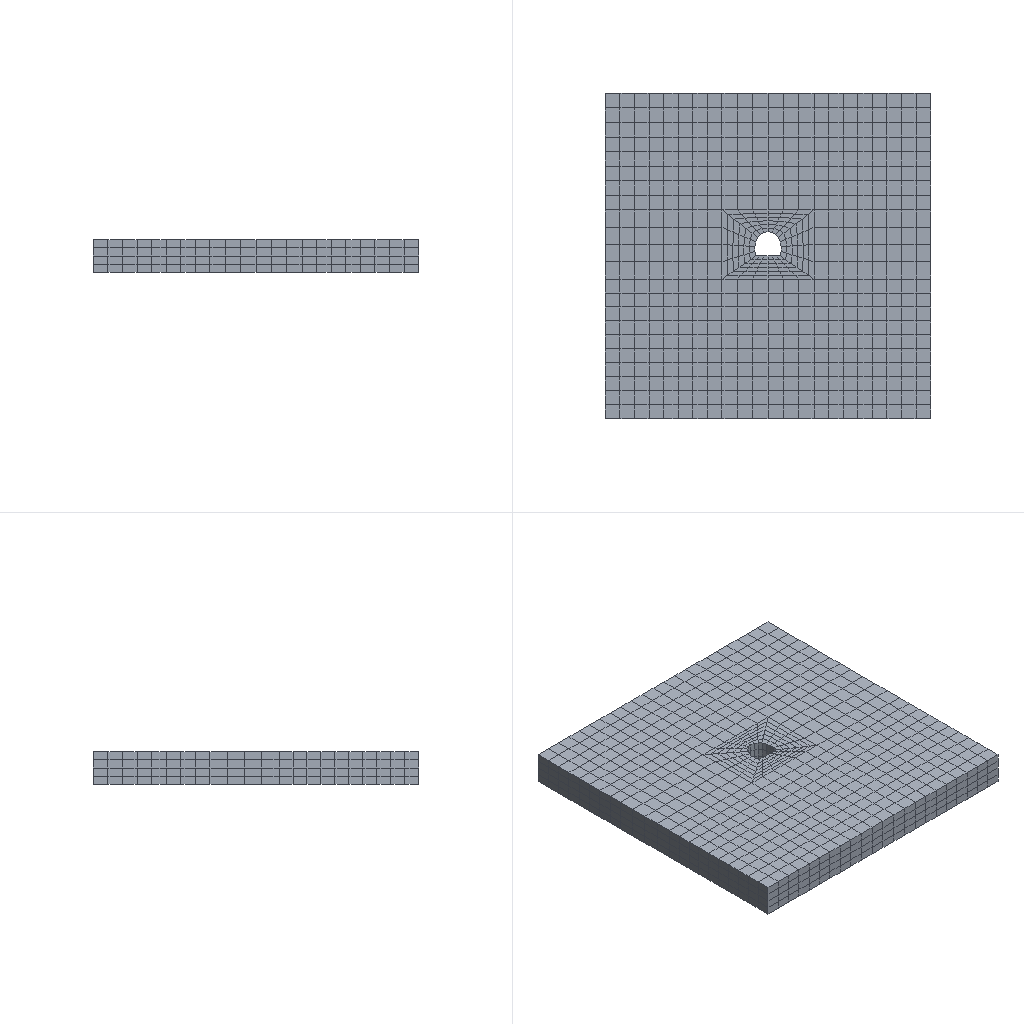Simulation study | abaqus
Set-up summary:
category,name,step,type,value,unit,region
solver,abaqus
solver,version,,,Abaqus/Standard 2020
units,not stated in the deck,,not stated
analysis,deck,,geostatic,geostatic; soils
load_step,Step-1,Step-1,geostatic,nlgeom=False
load_step,Step-2,Step-2,soils,nlgeom=False
contact,interactions,,,general=0 pairs=0 ties=0
load_step,requested,,,2
mesh,nodes,,,3170
mesh,elements,,,2320
element_type,C3D8PT,,solid,2320
load,load commands in deck,,count,1
bc,support commands in deck,,count,4
material,MATERIAL-1,,in results
check,setup vs results,,match,"per instance, exact: element labels, types and connectivity; labels of the nodes the elements use; coordinates of those nodes at SINGLE_PRECISION in 1 of 1 instance(s)"
Abaqus input file, long lists of numbers shortened:
*Heading
** Job name: Job-1 Model name: Job-try7
** Generated by: Abaqus/CAE 2020
*Preprint, echo=NO, model=NO, history=NO, contact=NO
**
** PARTS
**
*Part, name=PART-2
*Node
      1,   14.16,  -7.097,           0.
      2,   14.16,         -50.,           0.
** (3168 more lines like these left out)
*Element, type=C3D8PT
   1,  102,  597, 1893,  567,    1,   41,  477,   68
   2,  597,  598, 1894, 1893,   41,   42,  478,  477
** (2318 more lines like these left out)
*Nset, nset=_PICKEDSET2, internal, generate
    1,  3170,     1
*Elset, elset=_PICKEDSET2, internal, generate
    1,  2320,     1
** Section: Section-1-_PICKEDSET2
*Solid Section, elset=_PICKEDSET2, material=MATERIAL-1
,
*End Part
**
**
** ASSEMBLY
**
*Assembly, name=Assembly
**
*Instance, name=PART-2-1, part=PART-2
*End Instance
**
*Nset, nset=Set-12, instance=PART-2-1, generate
    1,  3170,     1
*Nset, nset=Set-13, instance=PART-2-1
   10,   11,   13,   14,   25,   26,   27,   28,  114,  115,  116,  130,  131,  132,  151,  152
  153,  154,  155,  156,  157,  158,  159,  160,  260,  261,  262,  268,  269,  270,  271,  272
** (5 more lines like these left out)
*Nset, nset=Set-14, instance=PART-2-1
   10,   11,   13,   14,   25,   26,   27,   28,  114,  115,  116,  130,  131,  132,  151,  152
  153,  154,  155,  156,  157,  158,  159,  160,  260,  261,  262,  268,  269,  270,  271,  272
** (5 more lines like these left out)
*Nset, nset=Set-15, instance=PART-2-1, generate
    1,  3170,     1
*Nset, nset=Set-16, instance=PART-2-1
   29,   30,   31,   32,   35,   36,   37,   38,  299,  300,  301,  302,  303,  304,  305,  306
  307,  308,  309,  310,  356,  357,  358,  359,  360,  361,  362,  363,  364,  365,  366,  367
** (6 more lines like these left out)
*Nset, nset=Set-17, instance=PART-2-1
    2,    3,    5,    6,   37,   38,   39,   40,   50,   51,   52,   53,   54,   78,   79,   80
   81,   82,  103,  104,  105,  106,  107,  108,  396,  397,  398,  408,  409,  410,  411,  412
** (6 more lines like these left out)
*Nset, nset=Set-18, instance=PART-2-1
    1,    2,    3,    4,    9,   10,   13,   16,   17,   18,   21,   24,   25,   27,   29,   30
   33,   35,   37,   39,   41,   42,   43,   44,   45,   46,   47,   48,   49,   50,   51,   52
** (38 more lines like these left out)
*Nset, nset=Set-19, instance=PART-2-1, generate
    1,  3170,     1
*Nset, nset=Set-20, instance=PART-2-1
    2,    3,    5,    6,   17,   18,   19,   20,   21,   22,   23,   24,   29,   30,   31,   32
   33,   34,   35,   36,   37,   38,   39,   40,   50,   51,   52,   53,   54,   78,   79,   80
** (26 more lines like these left out)
*Nset, nset=Set-21, instance=PART-2-1
   10,   11,   13,   14,   25,   26,   27,   28,  114,  115,  116,  130,  131,  132,  151,  152
  153,  154,  155,  156,  157,  158,  159,  160,  260,  261,  262,  268,  269,  270,  271,  272
** (5 more lines like these left out)
*Nset, nset=Set-22, instance=PART-2-1
    1,    2,    3,    4,    5,    6,    7,    8,    9,   10,   11,   12,   13,   14,   15,   16
   17,   18,   19,   20,   21,   22,   23,   24,   25,   26,   27,   28,   29,   30,   31,   32
** (78 more lines like these left out)
*Nset, nset=Set-23, instance=PART-2-1
    2,    3,    5,    6,   21,   22,   23,   24,   33,   34,   35,   36,   37,   38,   39,   40
   50,   51,   52,   53,   54,   78,   79,   80,   81,   82,  103,  104,  105,  106,  107,  108
** (13 more lines like these left out)
*Nset, nset=Set-24, instance=PART-2-1
   17,   18,   19,   20,   23,   24,   29,   30,   31,   32,   35,   36,   37,   38,   39,   40
  168,  169,  170,  188,  189,  190,  201,  202,  203,  204,  205,  206,  224,  225,  226,  227
** (13 more lines like these left out)
*Nset, nset=_PICKEDSET78, internal, instance=PART-2-1
   29,   30,   31,   32,   35,   36,   37,   38,  299,  300,  301,  302,  303,  304,  305,  306
  307,  308,  309,  310,  356,  357,  358,  359,  360,  361,  362,  363,  364,  365,  366,  367
** (6 more lines like these left out)
*Elset, elset=_PICKEDSET78, internal, instance=PART-2-1
 1073, 1074, 1075, 1076, 1077, 1078, 1079, 1080, 1081, 1082, 1083, 1084, 1085, 1086, 1087, 1088
 1313, 1314, 1315, 1316, 1317, 1318, 1319, 1320, 1321, 1322, 1323, 1324, 1325, 1326, 1327, 1328
** (4 more lines like these left out)
*Nset, nset=_PICKEDSET85, internal, instance=PART-2-1
    1,    2,    3,    4,    9,   10,   13,   16,   17,   18,   21,   24,   25,   27,   29,   30
   33,   35,   37,   39,   41,   42,   43,   44,   45,   46,   47,   48,   49,   50,   51,   52
** (38 more lines like these left out)
*Elset, elset=_PICKEDSET85, internal, instance=PART-2-1
    1,    2,    3,    4,    5,    6,    7,    8,    9,   10,   11,   12,   13,   14,   15,   16
   17,   18,   19,   20,   21,   22,   23,   24,   25,   26,   27,   28,   29,   30,   31,   32
** (35 more lines like these left out)
*Nset, nset=_PICKEDSET86, internal, instance=PART-2-1
    2,    3,    5,    6,   37,   38,   39,   40,   50,   51,   52,   53,   54,   78,   79,   80
   81,   82,  103,  104,  105,  106,  107,  108,  396,  397,  398,  408,  409,  410,  411,  412
** (6 more lines like these left out)
*Elset, elset=_PICKEDSET86, internal, instance=PART-2-1
   10,   20,   30,   40,   50,   60,   70,   80,   90,  100,  110,  120,  130,  140,  150,  160
  170,  180,  190,  200,  210,  220,  230,  240, 1381, 1382, 1383, 1384, 1421, 1422, 1423, 1424
** (4 more lines like these left out)
*Elset, elset=__PICKEDSURF74_S2, internal, instance=PART-2-1, generate
 1665,  1688,     1
*Elset, elset=__PICKEDSURF74_S6, internal, instance=PART-2-1
  513,  521,  529,  537,  545,  553,  561,  569,  577,  585,  593,  601,  609,  617,  625,  633
  641,  649,  657,  665,  673,  681,  689,  697,  705,  713,  721,  729,  737,  745,  753,  761
** (2 more lines like these left out)
*Elset, elset=__PICKEDSURF75_S1, internal, instance=PART-2-1
  737,  738,  739,  740,  741,  742,  743,  744,  745,  746,  747,  748,  749,  750,  751,  752
  753,  754,  755,  756,  757,  758,  759,  760,  761,  762,  763,  764,  765,  766,  767,  768
** (3 more lines like these left out)
*Elset, elset=__PICKEDSURF75_S4, internal, instance=PART-2-1, generate
 392,  512,    8
*Elset, elset=__PICKEDSURF84_S1, internal, instance=PART-2-1
 181, 182, 183, 184, 185, 186, 187, 188, 189, 190, 191, 192, 193, 194, 195, 196
 197, 198, 199, 200, 201, 202, 203, 204, 205, 206, 207, 208, 209, 210, 211, 212
** (4 more lines like these left out)
*Elset, elset=__PICKEDSURF84_S3, internal, instance=PART-2-1
 1857, 1858, 1859, 1860, 1861, 1862, 1881, 1882, 1883, 1884, 1885, 1886, 1905, 1906, 1907, 1908
 1909, 1910, 1929, 1930, 1931, 1932, 1933, 1934, 1953, 1954, 1955, 1956, 1957, 1958, 1977, 1978
** (1 more lines like these left out)
*Elset, elset=__PICKEDSURF84_S5, internal, instance=PART-2-1
  259,  260,  261,  262,  263,  264,  283,  284,  285,  286,  287,  288,  307,  308,  309,  310
  311,  312,  331,  332,  333,  334,  335,  336,  355,  356,  357,  358,  359,  360,  379,  380
** (19 more lines like these left out)
*Elset, elset=__PICKEDSURF84_S6, internal, instance=PART-2-1, generate
 1345,  1853,     4
*Elset, elset=__PICKEDSURF74_S6_1, internal, instance=PART-2-1
  513,  521,  529,  537,  545,  553,  561,  569,  577,  585,  593,  601,  609,  617,  625,  633
  641,  649,  657,  665,  673,  681,  689,  697,  705,  713,  721,  729,  737,  745,  753,  761
** (2 more lines like these left out)
*Elset, elset=__PICKEDSURF74_S2_1, internal, instance=PART-2-1, generate
 1665,  1688,     1
*Surface, type=ELEMENT, name=_PICKEDSURF74, internal
__PICKEDSURF74_S6_1, S6
__PICKEDSURF74_S2_1, S2
*Elset, elset=__PICKEDSURF75_S1_1, internal, instance=PART-2-1
  737,  738,  739,  740,  741,  742,  743,  744,  745,  746,  747,  748,  749,  750,  751,  752
  753,  754,  755,  756,  757,  758,  759,  760,  761,  762,  763,  764,  765,  766,  767,  768
** (3 more lines like these left out)
*Elset, elset=__PICKEDSURF75_S4_1, internal, instance=PART-2-1, generate
 392,  512,    8
*Surface, type=ELEMENT, name=_PICKEDSURF75, internal
__PICKEDSURF75_S1_1, S1
__PICKEDSURF75_S4_1, S4
*Elset, elset=__PICKEDSURF84_S6_1, internal, instance=PART-2-1, generate
 1345,  1853,     4
*Elset, elset=__PICKEDSURF84_S5_1, internal, instance=PART-2-1
  259,  260,  261,  262,  263,  264,  283,  284,  285,  286,  287,  288,  307,  308,  309,  310
  311,  312,  331,  332,  333,  334,  335,  336,  355,  356,  357,  358,  359,  360,  379,  380
** (19 more lines like these left out)
*Elset, elset=__PICKEDSURF84_S1_1, internal, instance=PART-2-1
 181, 182, 183, 184, 185, 186, 187, 188, 189, 190, 191, 192, 193, 194, 195, 196
 197, 198, 199, 200, 201, 202, 203, 204, 205, 206, 207, 208, 209, 210, 211, 212
** (4 more lines like these left out)
*Elset, elset=__PICKEDSURF84_S3_1, internal, instance=PART-2-1
 1857, 1858, 1859, 1860, 1861, 1862, 1881, 1882, 1883, 1884, 1885, 1886, 1905, 1906, 1907, 1908
 1909, 1910, 1929, 1930, 1931, 1932, 1933, 1934, 1953, 1954, 1955, 1956, 1957, 1958, 1977, 1978
** (1 more lines like these left out)
*Surface, type=ELEMENT, name=_PICKEDSURF84, internal
__PICKEDSURF84_S6_1, S6
__PICKEDSURF84_S5_1, S5
__PICKEDSURF84_S1_1, S1
__PICKEDSURF84_S3_1, S3
*End Assembly
**
** MATERIALS
**
*Material, name=MATERIAL-1
*Conductivity
1000.,
*Density
2700.,
*Elastic
 5e+10, 0.3
*Expansion
 1e-06,
*Permeability, specific=9800.
 1e-07, 0.2
*Specific Heat
780.,
**
** PREDEFINED FIELDS
**
** Name: Predefined Field-1   Type: Void ratio
*Initial Conditions, TYPE=RATIO
Set-12, 0.2
** Name: Predefined Field-3   Type: Pore pressure
*Initial Conditions, TYPE=PORE PRESSURE
Set-15, 1e+06
** Name: Predefined Field-4   Type: Temperature
*Initial Conditions, type=TEMPERATURE
Set-19, 50.
** ----------------------------------------------------------------
**
** STEP: Step-1
**
*Step, name=Step-1, nlgeom=NO, inc=1000, unsymm=YES
*Geostatic
**
** BOUNDARY CONDITIONS
**
** Name: BC-11 Type: 位移/转角
*Boundary
Set-22, 3, 3
** Name: BC-12 Type: 位移/转角
*Boundary
Set-23, 2, 2
** Name: BC-13 Type: 位移/转角
*Boundary
Set-24, 1, 1
**
** OUTPUT REQUESTS
**
*Restart, write, frequency=0
**
** FIELD OUTPUT: F-Output-1
**
*Output, field
*Node Output
CF, NT, POR, RF, RM, RT, TF, U
V
*Element Output, directions=YES
E, FLUVR, FLVEL, GELVR, LE, MISES, MISESMAX, MISESONLY, NE, PE, PEEQ, PEEQMAX, PEEQT, PEMAG, PRESSONLY, S
SAT, SEQUT, SF, SROCK, SSAVG, TEMP, VOIDR, YIELDPOT
*Contact Output
CDISP, CSTRESS
**
** HISTORY OUTPUT: H-Output-1
**
*Output, history, variable=PRESELECT
*End Step
** ----------------------------------------------------------------
**
** STEP: Step-2
**
*Step, name=Step-2, nlgeom=NO, inc=10000, unsymm=YES
*Soils, consolidation, end=PERIOD, utol=1e+13, creep=none
10., 100000., 1., 1000.,
**
** BOUNDARY CONDITIONS
**
** Name: BC-7 Type: 温度
*Boundary
Set-21, 11, 11, 5.
**
** OUTPUT REQUESTS
**
*Restart, write, frequency=0
**
** FIELD OUTPUT: F-Output-1
**
*Output, field
*Node Output
CF, NT, POR, RF, RM, RT, TF, U
V
*Element Output, directions=YES
E, FLUVR, FLVEL, GELVR, LE, MISES, MISESMAX, MISESONLY, NE, PE, PEEQ, PEEQMAX, PEEQT, PEMAG, PRESSONLY, S
SAT, SEQUT, SF, SROCK, SSAVG, TEMP, VOIDR, YIELDPOT
*Contact Output
CDISP, CSTRESS
**
** HISTORY OUTPUT: H-Output-1
**
*Output, history, variable=PRESELECT
*End Step
Results summary:
result,step,,completed,increments=1 time=1.0/1.0
result,step,,completed,increments=112 time=100000.0/100000.0
result,analysis,,,"soils, consolidation"
result,last_loadstep,,,2
result,analysis steps,,count,2
result,primary field,,,"U, POR"
result,reaction total,,FX,0.0,model units
result,reaction total,,FY,-64.0,model units
result,reaction total,,FZ,0.0,model units